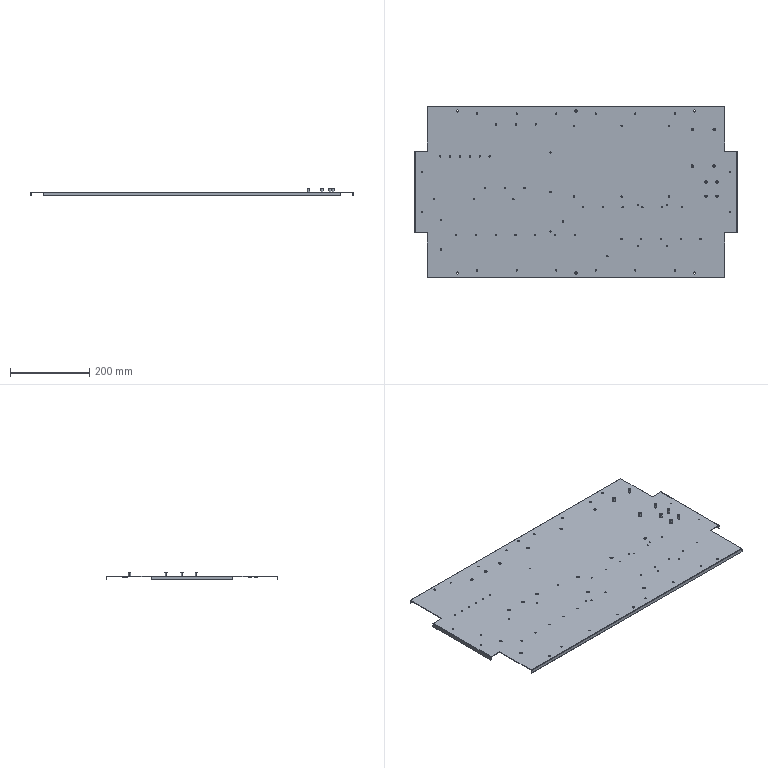Part | STEP file | component mounting plate | 1 solid | 278 faces | box 817 x 435 x 20 mm | volume 536830 mm3 | cylinder 216 | plane 62 | commonest cylinder face diameters 3.3 x132 8 x32 2.5 x16 6 x16 5.5 x12 0.02 x4